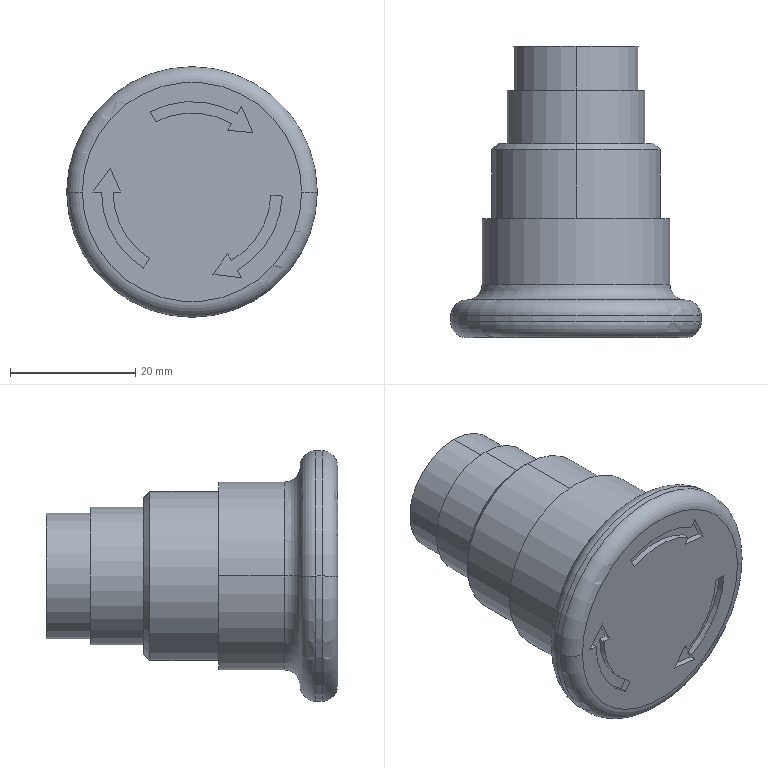Part | SolidWorks | features BaseBody 1 | 1 solid | 50 faces | box 40 x 46.5 x 40 mm | volume 27930 mm3 | plane 24 | cylinder 18 | torus 6 | cone 2 | commonest cylinder face diameters 25.213 x3 28.872 x3 18 x2 20 x2 22 x2 27 x2
STEP:
#1=CARTESIAN_POINT('',(14.421,1.,-0.6518));
#2=VERTEX_POINT('',#1);
#3=CARTESIAN_POINT('',(12.594,1.,-0.5692));
#4=VERTEX_POINT('',#3);
#5=CARTESIAN_POINT('',(14.421,1.,-0.6518));
#6=DIRECTION('',(-0.999,0.,0.04515));
#7=VECTOR('',#6,1000.);
#8=LINE('',#5,#7);
#9=EDGE_CURVE('',#2,#4,#8,.T.);
#10=ORIENTED_EDGE('',*,*,#9,.T.);
#11=CARTESIAN_POINT('',(6.303,1.,-10.918));
#12=VERTEX_POINT('',#11);
#13=CARTESIAN_POINT('',(0.,1.,0.));
#14=DIRECTION('',(0.,1.,0.));
#15=DIRECTION('',(0.999,0.,-0.04515));
#16=AXIS2_PLACEMENT_3D('',#13,#14,#15);
#17=CIRCLE('',#16,12.607);
#18=EDGE_CURVE('',#4,#12,#17,.T.);
#19=ORIENTED_EDGE('',*,*,#18,.T.);
#20=CARTESIAN_POINT('',(5.687,1.,-9.849));
#21=VERTEX_POINT('',#20);
#22=CARTESIAN_POINT('',(6.303,1.,-10.918));
#23=DIRECTION('',(-0.5,0.,0.866));
#24=VECTOR('',#23,1000.);
#25=LINE('',#22,#24);
#26=EDGE_CURVE('',#12,#21,#25,.T.);
#27=ORIENTED_EDGE('',*,*,#26,.T.);
#28=CARTESIAN_POINT('',(3.346,1.,-13.147));
#29=VERTEX_POINT('',#28);
#30=CARTESIAN_POINT('',(5.687,1.,-9.849));
#31=DIRECTION('',(-0.5788,0.,-0.8155));
#32=VECTOR('',#31,1000.);
#33=LINE('',#30,#32);
#34=EDGE_CURVE('',#21,#29,#33,.T.);
#35=ORIENTED_EDGE('',*,*,#34,.T.);
#36=CARTESIAN_POINT('',(7.903,1.,-13.688));
#37=VERTEX_POINT('',#36);
#38=CARTESIAN_POINT('',(3.346,1.,-13.147));
#39=DIRECTION('',(0.993,0.,-0.1179));
#40=VECTOR('',#39,1000.);
#41=LINE('',#38,#40);
#42=EDGE_CURVE('',#29,#37,#41,.T.);
#43=ORIENTED_EDGE('',*,*,#42,.T.);
#44=CARTESIAN_POINT('',(7.218,1.,-12.502));
#45=VERTEX_POINT('',#44);
#46=CARTESIAN_POINT('',(7.903,1.,-13.688));
#47=DIRECTION('',(-0.5,0.,0.866));
#48=VECTOR('',#47,1000.);
#49=LINE('',#46,#48);
#50=EDGE_CURVE('',#37,#45,#49,.T.);
#51=ORIENTED_EDGE('',*,*,#50,.T.);
#52=CARTESIAN_POINT('',(0.,1.,0.));
#53=DIRECTION('',(0.,-1.,0.));
#54=DIRECTION('',(0.5,0.,-0.866));
#55=AXIS2_PLACEMENT_3D('',#52,#53,#54);
#56=CIRCLE('',#55,14.436);
#57=EDGE_CURVE('',#45,#2,#56,.T.);
#58=ORIENTED_EDGE('',*,*,#57,.T.);
#59=EDGE_LOOP('',(#10,#19,#27,#35,#43,#51,#58));
#60=FACE_OUTER_BOUND('',#59,.T.);
#61=CARTESIAN_POINT('',(0.,1.,0.));
#62=DIRECTION('',(0.,-1.,0.));
#63=DIRECTION('',(-0.866,0.,-0.5));
#64=AXIS2_PLACEMENT_3D('',#61,#62,#63);
#65=PLANE('',#64);
#66=ADVANCED_FACE('',(#60),#65,.T.);
#67=CARTESIAN_POINT('',(12.594,0.,-0.5692));
#68=VERTEX_POINT('',#67);
#69=CARTESIAN_POINT('',(12.594,0.,-0.5692));
#70=DIRECTION('',(0.,1.,0.));
#71=VECTOR('',#70,1000.);
#72=LINE('',#69,#71);
#73=EDGE_CURVE('',#68,#4,#72,.T.);
#74=ORIENTED_EDGE('',*,*,#73,.T.);
#75=ORIENTED_EDGE('',*,*,#9,.F.);
#76=CARTESIAN_POINT('',(14.421,0.,-0.6518));
#77=VERTEX_POINT('',#76);
#78=CARTESIAN_POINT('',(14.421,0.,-0.6518));
#79=DIRECTION('',(0.,1.,0.));
#80=VECTOR('',#79,1000.);
#81=LINE('',#78,#80);
#82=EDGE_CURVE('',#77,#2,#81,.T.);
#83=ORIENTED_EDGE('',*,*,#82,.F.);
#84=CARTESIAN_POINT('',(14.421,0.,-0.6518));
#85=DIRECTION('',(-0.999,0.,0.04515));
#86=VECTOR('',#85,1000.);
#87=LINE('',#84,#86);
#88=EDGE_CURVE('',#77,#68,#87,.T.);
#89=ORIENTED_EDGE('',*,*,#88,.T.);
#90=EDGE_LOOP('',(#74,#75,#83,#89));
#91=FACE_OUTER_BOUND('',#90,.T.);
#92=CARTESIAN_POINT('',(14.421,0.,-0.6518));
#93=DIRECTION('',(0.04515,0.,0.999));
#94=DIRECTION('',(-0.999,0.,0.04515));
#95=AXIS2_PLACEMENT_3D('',#92,#93,#94);
#96=PLANE('',#95);
#97=ADVANCED_FACE('',(#91),#96,.F.);
#98=CARTESIAN_POINT('',(6.303,0.,-10.918));
#99=VERTEX_POINT('',#98);
#100=CARTESIAN_POINT('',(6.303,0.,-10.918));
#101=DIRECTION('',(0.,1.,0.));
#102=VECTOR('',#101,1000.);
#103=LINE('',#100,#102);
#104=EDGE_CURVE('',#99,#12,#103,.T.);
#105=ORIENTED_EDGE('',*,*,#104,.T.);
#106=ORIENTED_EDGE('',*,*,#18,.F.);
#107=ORIENTED_EDGE('',*,*,#73,.F.);
#108=CARTESIAN_POINT('',(0.,0.,0.));
#109=DIRECTION('',(0.,-1.,0.));
#110=DIRECTION('',(0.5,0.,-0.866));
#111=AXIS2_PLACEMENT_3D('',#108,#109,#110);
#112=CIRCLE('',#111,12.607);
#113=EDGE_CURVE('',#99,#68,#112,.T.);
#114=ORIENTED_EDGE('',*,*,#113,.F.);
#115=EDGE_LOOP('',(#105,#106,#107,#114));
#116=FACE_OUTER_BOUND('',#115,.T.);
#117=CARTESIAN_POINT('',(0.,0.,0.));
#118=DIRECTION('',(0.,-1.,0.));
#119=DIRECTION('',(-0.866,0.,-0.5));
#120=AXIS2_PLACEMENT_3D('',#117,#118,#119);
#121=CYLINDRICAL_SURFACE('',#120,12.607);
#122=ADVANCED_FACE('',(#116),#121,.T.);
#123=CARTESIAN_POINT('',(5.687,0.,-9.849));
#124=VERTEX_POINT('',#123);
#125=CARTESIAN_POINT('',(5.687,0.,-9.849));
#126=DIRECTION('',(0.,1.,0.));
#127=VECTOR('',#126,1000.);
#128=LINE('',#125,#127);
#129=EDGE_CURVE('',#124,#21,#128,.T.);
#130=ORIENTED_EDGE('',*,*,#129,.T.);
#131=ORIENTED_EDGE('',*,*,#26,.F.);
#132=ORIENTED_EDGE('',*,*,#104,.F.);
#133=CARTESIAN_POINT('',(6.303,0.,-10.918));
#134=DIRECTION('',(-0.5,0.,0.866));
#135=VECTOR('',#134,1000.);
#136=LINE('',#133,#135);
#137=EDGE_CURVE('',#99,#124,#136,.T.);
#138=ORIENTED_EDGE('',*,*,#137,.T.);
#139=EDGE_LOOP('',(#130,#131,#132,#138));
#140=FACE_OUTER_BOUND('',#139,.T.);
#141=CARTESIAN_POINT('',(6.303,0.,-10.918));
#142=DIRECTION('',(0.866,0.,0.5));
#143=DIRECTION('',(-0.5,0.,0.866));
#144=AXIS2_PLACEMENT_3D('',#141,#142,#143);
#145=PLANE('',#144);
#146=ADVANCED_FACE('',(#140),#145,.F.);
#147=CARTESIAN_POINT('',(3.346,0.,-13.147));
#148=VERTEX_POINT('',#147);
#149=CARTESIAN_POINT('',(3.346,0.,-13.147));
#150=DIRECTION('',(0.,1.,0.));
#151=VECTOR('',#150,1000.);
#152=LINE('',#149,#151);
#153=EDGE_CURVE('',#148,#29,#152,.T.);
#154=ORIENTED_EDGE('',*,*,#153,.T.);
#155=ORIENTED_EDGE('',*,*,#34,.F.);
#156=ORIENTED_EDGE('',*,*,#129,.F.);
#157=CARTESIAN_POINT('',(5.687,0.,-9.849));
#158=DIRECTION('',(-0.5788,0.,-0.8155));
#159=VECTOR('',#158,1000.);
#160=LINE('',#157,#159);
#161=EDGE_CURVE('',#124,#148,#160,.T.);
#162=ORIENTED_EDGE('',*,*,#161,.T.);
#163=EDGE_LOOP('',(#154,#155,#156,#162));
#164=FACE_OUTER_BOUND('',#163,.T.);
#165=CARTESIAN_POINT('',(5.687,0.,-9.849));
#166=DIRECTION('',(-0.8155,0.,0.5788));
#167=DIRECTION('',(-0.5788,0.,-0.8155));
#168=AXIS2_PLACEMENT_3D('',#165,#166,#167);
#169=PLANE('',#168);
#170=ADVANCED_FACE('',(#164),#169,.F.);
#171=CARTESIAN_POINT('',(7.903,0.,-13.688));
#172=VERTEX_POINT('',#171);
#173=CARTESIAN_POINT('',(7.903,0.,-13.688));
#174=DIRECTION('',(0.,1.,0.));
#175=VECTOR('',#174,1000.);
#176=LINE('',#173,#175);
#177=EDGE_CURVE('',#172,#37,#176,.T.);
#178=ORIENTED_EDGE('',*,*,#177,.T.);
#179=ORIENTED_EDGE('',*,*,#42,.F.);
#180=ORIENTED_EDGE('',*,*,#153,.F.);
#181=CARTESIAN_POINT('',(3.346,0.,-13.147));
#182=DIRECTION('',(0.993,0.,-0.1179));
#183=VECTOR('',#182,1000.);
#184=LINE('',#181,#183);
#185=EDGE_CURVE('',#148,#172,#184,.T.);
#186=ORIENTED_EDGE('',*,*,#185,.T.);
#187=EDGE_LOOP('',(#178,#179,#180,#186));
#188=FACE_OUTER_BOUND('',#187,.T.);
#189=CARTESIAN_POINT('',(3.346,0.,-13.147));
#190=DIRECTION('',(-0.1179,0.,-0.993));
#191=DIRECTION('',(0.993,0.,-0.1179));
#192=AXIS2_PLACEMENT_3D('',#189,#190,#191);
#193=PLANE('',#192);
#194=ADVANCED_FACE('',(#188),#193,.F.);
#195=CARTESIAN_POINT('',(7.218,0.,-12.502));
#196=VERTEX_POINT('',#195);
#197=CARTESIAN_POINT('',(7.218,0.,-12.502));
#198=DIRECTION('',(0.,1.,0.));
#199=VECTOR('',#198,1000.);
#200=LINE('',#197,#199);
#201=EDGE_CURVE('',#196,#45,#200,.T.);
#202=ORIENTED_EDGE('',*,*,#201,.T.);
#203=ORIENTED_EDGE('',*,*,#50,.F.);
#204=ORIENTED_EDGE('',*,*,#177,.F.);
#205=CARTESIAN_POINT('',(7.903,0.,-13.688));
#206=DIRECTION('',(-0.5,0.,0.866));
#207=VECTOR('',#206,1000.);
#208=LINE('',#205,#207);
#209=EDGE_CURVE('',#172,#196,#208,.T.);
#210=ORIENTED_EDGE('',*,*,#209,.T.);
#211=EDGE_LOOP('',(#202,#203,#204,#210));
#212=FACE_OUTER_BOUND('',#211,.T.);
#213=CARTESIAN_POINT('',(7.903,0.,-13.688));
#214=DIRECTION('',(0.866,0.,0.5));
#215=DIRECTION('',(-0.5,0.,0.866));
#216=AXIS2_PLACEMENT_3D('',#213,#214,#215);
#217=PLANE('',#216);
#218=ADVANCED_FACE('',(#212),#217,.F.);
#219=ORIENTED_EDGE('',*,*,#82,.T.);
#220=ORIENTED_EDGE('',*,*,#57,.F.);
#221=ORIENTED_EDGE('',*,*,#201,.F.);
#222=CARTESIAN_POINT('',(0.,0.,0.));
#223=DIRECTION('',(0.,-1.,0.));
#224=DIRECTION('',(0.5,0.,-0.866));
#225=AXIS2_PLACEMENT_3D('',#222,#223,#224);
#226=CIRCLE('',#225,14.436);
#227=EDGE_CURVE('',#196,#77,#226,.T.);
#228=ORIENTED_EDGE('',*,*,#227,.T.);
#229=EDGE_LOOP('',(#219,#220,#221,#228));
#230=FACE_OUTER_BOUND('',#229,.T.);
#231=CARTESIAN_POINT('',(0.,0.,0.));
#232=DIRECTION('',(0.,-1.,0.));
#233=DIRECTION('',(-0.866,0.,-0.5));
#234=AXIS2_PLACEMENT_3D('',#231,#232,#233);
#235=CYLINDRICAL_SURFACE('',#234,14.436);
#236=ADVANCED_FACE('',(#230),#235,.F.);
#237=CARTESIAN_POINT('',(-6.646,1.,12.815));
#238=VERTEX_POINT('',#237);
#239=CARTESIAN_POINT('',(-5.804,1.,11.191));
#240=VERTEX_POINT('',#239);
#241=CARTESIAN_POINT('',(-6.646,1.,12.815));
#242=DIRECTION('',(0.4604,0.,-0.8877));
#243=VECTOR('',#242,1000.);
#244=LINE('',#241,#243);
#245=EDGE_CURVE('',#238,#240,#244,.T.);
#246=ORIENTED_EDGE('',*,*,#245,.T.);
#247=CARTESIAN_POINT('',(6.303,1.,10.918));
#248=VERTEX_POINT('',#247);
#249=CARTESIAN_POINT('',(0.,1.,0.));
#250=DIRECTION('',(0.,1.,0.));
#251=DIRECTION('',(-0.4604,0.,0.8877));
#252=AXIS2_PLACEMENT_3D('',#249,#250,#251);
#253=CIRCLE('',#252,12.607);
#254=EDGE_CURVE('',#240,#248,#253,.T.);
#255=ORIENTED_EDGE('',*,*,#254,.T.);
#256=CARTESIAN_POINT('',(5.687,1.,9.849));
#257=VERTEX_POINT('',#256);
#258=CARTESIAN_POINT('',(6.303,1.,10.918));
#259=DIRECTION('',(-0.5,0.,-0.866));
#260=VECTOR('',#259,1000.);
#261=LINE('',#258,#260);
#262=EDGE_CURVE('',#248,#257,#261,.T.);
#263=ORIENTED_EDGE('',*,*,#262,.T.);
#264=CARTESIAN_POINT('',(9.712,1.,9.471));
#265=VERTEX_POINT('',#264);
#266=CARTESIAN_POINT('',(5.687,1.,9.849));
#267=DIRECTION('',(0.9956,0.,-0.09348));
#268=VECTOR('',#267,1000.);
#269=LINE('',#266,#268);
#270=EDGE_CURVE('',#257,#265,#269,.T.);
#271=ORIENTED_EDGE('',*,*,#270,.T.);
#272=CARTESIAN_POINT('',(7.903,1.,13.688));
#273=VERTEX_POINT('',#272);
#274=CARTESIAN_POINT('',(9.712,1.,9.471));
#275=DIRECTION('',(-0.3944,0.,0.9189));
#276=VECTOR('',#275,1000.);
#277=LINE('',#274,#276);
#278=EDGE_CURVE('',#265,#273,#277,.T.);
#279=ORIENTED_EDGE('',*,*,#278,.T.);
#280=CARTESIAN_POINT('',(7.218,1.,12.502));
#281=VERTEX_POINT('',#280);
#282=CARTESIAN_POINT('',(7.903,1.,13.688));
#283=DIRECTION('',(-0.5,0.,-0.866));
#284=VECTOR('',#283,1000.);
#285=LINE('',#282,#284);
#286=EDGE_CURVE('',#273,#281,#285,.T.);
#287=ORIENTED_EDGE('',*,*,#286,.T.);
#288=CARTESIAN_POINT('',(0.,1.,0.));
#289=DIRECTION('',(0.,-1.,0.));
#290=DIRECTION('',(0.5,0.,0.866));
#291=AXIS2_PLACEMENT_3D('',#288,#289,#290);
#292=CIRCLE('',#291,14.436);
#293=EDGE_CURVE('',#281,#238,#292,.T.);
#294=ORIENTED_EDGE('',*,*,#293,.T.);
#295=EDGE_LOOP('',(#246,#255,#263,#271,#279,#287,#294));
#296=FACE_OUTER_BOUND('',#295,.T.);
#297=CARTESIAN_POINT('',(0.,1.,0.));
#298=DIRECTION('',(0.,-1.,0.));
#299=DIRECTION('',(0.866,0.,-0.5));
#300=AXIS2_PLACEMENT_3D('',#297,#298,#299);
#301=PLANE('',#300);
#302=ADVANCED_FACE('',(#296),#301,.T.);
#303=CARTESIAN_POINT('',(-5.804,0.,11.191));
#304=VERTEX_POINT('',#303);
#305=CARTESIAN_POINT('',(-5.804,0.,11.191));
#306=DIRECTION('',(0.,1.,0.));
#307=VECTOR('',#306,1000.);
#308=LINE('',#305,#307);
#309=EDGE_CURVE('',#304,#240,#308,.T.);
#310=ORIENTED_EDGE('',*,*,#309,.T.);
#311=ORIENTED_EDGE('',*,*,#245,.F.);
#312=CARTESIAN_POINT('',(-6.646,0.,12.815));
#313=VERTEX_POINT('',#312);
#314=CARTESIAN_POINT('',(-6.646,0.,12.815));
#315=DIRECTION('',(0.,1.,0.));
#316=VECTOR('',#315,1000.);
#317=LINE('',#314,#316);
#318=EDGE_CURVE('',#313,#238,#317,.T.);
#319=ORIENTED_EDGE('',*,*,#318,.F.);
#320=CARTESIAN_POINT('',(-6.646,0.,12.815));
#321=DIRECTION('',(0.4604,0.,-0.8877));
#322=VECTOR('',#321,1000.);
#323=LINE('',#320,#322);
#324=EDGE_CURVE('',#313,#304,#323,.T.);
#325=ORIENTED_EDGE('',*,*,#324,.T.);
#326=EDGE_LOOP('',(#310,#311,#319,#325));
#327=FACE_OUTER_BOUND('',#326,.T.);
#328=CARTESIAN_POINT('',(-6.646,0.,12.815));
#329=DIRECTION('',(-0.8877,0.,-0.4604));
#330=DIRECTION('',(0.4604,0.,-0.8877));
#331=AXIS2_PLACEMENT_3D('',#328,#329,#330);
#332=PLANE('',#331);
#333=ADVANCED_FACE('',(#327),#332,.F.);
#334=CARTESIAN_POINT('',(6.303,0.,10.918));
#335=VERTEX_POINT('',#334);
#336=CARTESIAN_POINT('',(6.303,0.,10.918));
#337=DIRECTION('',(0.,1.,0.));
#338=VECTOR('',#337,1000.);
#339=LINE('',#336,#338);
#340=EDGE_CURVE('',#335,#248,#339,.T.);
#341=ORIENTED_EDGE('',*,*,#340,.T.);
#342=ORIENTED_EDGE('',*,*,#254,.F.);
#343=ORIENTED_EDGE('',*,*,#309,.F.);
#344=CARTESIAN_POINT('',(0.,0.,0.));
#345=DIRECTION('',(0.,-1.,0.));
#346=DIRECTION('',(0.5,0.,0.866));
#347=AXIS2_PLACEMENT_3D('',#344,#345,#346);
#348=CIRCLE('',#347,12.607);
#349=EDGE_CURVE('',#335,#304,#348,.T.);
#350=ORIENTED_EDGE('',*,*,#349,.F.);
#351=EDGE_LOOP('',(#341,#342,#343,#350));
#352=FACE_OUTER_BOUND('',#351,.T.);
#353=CARTESIAN_POINT('',(0.,0.,0.));
#354=DIRECTION('',(0.,-1.,0.));
#355=DIRECTION('',(0.866,0.,-0.5));
#356=AXIS2_PLACEMENT_3D('',#353,#354,#355);
#357=CYLINDRICAL_SURFACE('',#356,12.607);
#358=ADVANCED_FACE('',(#352),#357,.T.);
#359=CARTESIAN_POINT('',(5.687,0.,9.849));
#360=VERTEX_POINT('',#359);
#361=CARTESIAN_POINT('',(5.687,0.,9.849));
#362=DIRECTION('',(0.,1.,0.));
#363=VECTOR('',#362,1000.);
#364=LINE('',#361,#363);
#365=EDGE_CURVE('',#360,#257,#364,.T.);
#366=ORIENTED_EDGE('',*,*,#365,.T.);
#367=ORIENTED_EDGE('',*,*,#262,.F.);
#368=ORIENTED_EDGE('',*,*,#340,.F.);
#369=CARTESIAN_POINT('',(6.303,0.,10.918));
#370=DIRECTION('',(-0.5,0.,-0.866));
#371=VECTOR('',#370,1000.);
#372=LINE('',#369,#371);
#373=EDGE_CURVE('',#335,#360,#372,.T.);
#374=ORIENTED_EDGE('',*,*,#373,.T.);
#375=EDGE_LOOP('',(#366,#367,#368,#374));
#376=FACE_OUTER_BOUND('',#375,.T.);
#377=CARTESIAN_POINT('',(6.303,0.,10.918));
#378=DIRECTION('',(-0.866,0.,0.5));
#379=DIRECTION('',(-0.5,0.,-0.866));
#380=AXIS2_PLACEMENT_3D('',#377,#378,#379);
#381=PLANE('',#380);
#382=ADVANCED_FACE('',(#376),#381,.F.);
#383=CARTESIAN_POINT('',(9.712,0.,9.471));
#384=VERTEX_POINT('',#383);
#385=CARTESIAN_POINT('',(9.712,0.,9.471));
#386=DIRECTION('',(0.,1.,0.));
#387=VECTOR('',#386,1000.);
#388=LINE('',#385,#387);
#389=EDGE_CURVE('',#384,#265,#388,.T.);
#390=ORIENTED_EDGE('',*,*,#389,.T.);
#391=ORIENTED_EDGE('',*,*,#270,.F.);
#392=ORIENTED_EDGE('',*,*,#365,.F.);
#393=CARTESIAN_POINT('',(5.687,0.,9.849));
#394=DIRECTION('',(0.9956,0.,-0.09348));
#395=VECTOR('',#394,1000.);
#396=LINE('',#393,#395);
#397=EDGE_CURVE('',#360,#384,#396,.T.);
#398=ORIENTED_EDGE('',*,*,#397,.T.);
#399=EDGE_LOOP('',(#390,#391,#392,#398));
#400=FACE_OUTER_BOUND('',#399,.T.);
#401=CARTESIAN_POINT('',(5.687,0.,9.849));
#402=DIRECTION('',(-0.09348,0.,-0.9956));
#403=DIRECTION('',(0.9956,0.,-0.09348));
#404=AXIS2_PLACEMENT_3D('',#401,#402,#403);
#405=PLANE('',#404);
#406=ADVANCED_FACE('',(#400),#405,.F.);
#407=CARTESIAN_POINT('',(7.903,0.,13.688));
#408=VERTEX_POINT('',#407);
#409=CARTESIAN_POINT('',(7.903,0.,13.688));
#410=DIRECTION('',(0.,1.,0.));
#411=VECTOR('',#410,1000.);
#412=LINE('',#409,#411);
#413=EDGE_CURVE('',#408,#273,#412,.T.);
#414=ORIENTED_EDGE('',*,*,#413,.T.);
#415=ORIENTED_EDGE('',*,*,#278,.F.);
#416=ORIENTED_EDGE('',*,*,#389,.F.);
#417=CARTESIAN_POINT('',(9.712,0.,9.471));
#418=DIRECTION('',(-0.3944,0.,0.9189));
#419=VECTOR('',#418,1000.);
#420=LINE('',#417,#419);
#421=EDGE_CURVE('',#384,#408,#420,.T.);
#422=ORIENTED_EDGE('',*,*,#421,.T.);
#423=EDGE_LOOP('',(#414,#415,#416,#422));
#424=FACE_OUTER_BOUND('',#423,.T.);
#425=CARTESIAN_POINT('',(9.712,0.,9.471));
#426=DIRECTION('',(0.9189,0.,0.3944));
#427=DIRECTION('',(-0.3944,0.,0.9189));
#428=AXIS2_PLACEMENT_3D('',#425,#426,#427);
#429=PLANE('',#428);
#430=ADVANCED_FACE('',(#424),#429,.F.);
#431=CARTESIAN_POINT('',(7.218,0.,12.502));
#432=VERTEX_POINT('',#431);
#433=CARTESIAN_POINT('',(7.218,0.,12.502));
#434=DIRECTION('',(0.,1.,0.));
#435=VECTOR('',#434,1000.);
#436=LINE('',#433,#435);
#437=EDGE_CURVE('',#432,#281,#436,.T.);
#438=ORIENTED_EDGE('',*,*,#437,.T.);
#439=ORIENTED_EDGE('',*,*,#286,.F.);
#440=ORIENTED_EDGE('',*,*,#413,.F.);
#441=CARTESIAN_POINT('',(7.903,0.,13.688));
#442=DIRECTION('',(-0.5,0.,-0.866));
#443=VECTOR('',#442,1000.);
#444=LINE('',#441,#443);
#445=EDGE_CURVE('',#408,#432,#444,.T.);
#446=ORIENTED_EDGE('',*,*,#445,.T.);
#447=EDGE_LOOP('',(#438,#439,#440,#446));
#448=FACE_OUTER_BOUND('',#447,.T.);
#449=CARTESIAN_POINT('',(7.903,0.,13.688));
#450=DIRECTION('',(-0.866,0.,0.5));
#451=DIRECTION('',(-0.5,0.,-0.866));
#452=AXIS2_PLACEMENT_3D('',#449,#450,#451);
#453=PLANE('',#452);
#454=ADVANCED_FACE('',(#448),#453,.F.);
#455=ORIENTED_EDGE('',*,*,#318,.T.);
#456=ORIENTED_EDGE('',*,*,#293,.F.);
#457=ORIENTED_EDGE('',*,*,#437,.F.);
#458=CARTESIAN_POINT('',(0.,0.,0.));
#459=DIRECTION('',(0.,-1.,0.));
#460=DIRECTION('',(0.5,0.,0.866));
#461=AXIS2_PLACEMENT_3D('',#458,#459,#460);
#462=CIRCLE('',#461,14.436);
#463=EDGE_CURVE('',#432,#313,#462,.T.);
#464=ORIENTED_EDGE('',*,*,#463,.T.);
#465=EDGE_LOOP('',(#455,#456,#457,#464));
#466=FACE_OUTER_BOUND('',#465,.T.);
#467=CARTESIAN_POINT('',(0.,0.,0.));
#468=DIRECTION('',(0.,-1.,0.));
#469=DIRECTION('',(0.866,0.,-0.5));
#470=AXIS2_PLACEMENT_3D('',#467,#468,#469);
#471=CYLINDRICAL_SURFACE('',#470,14.436);
#472=ADVANCED_FACE('',(#466),#471,.F.);
#473=CARTESIAN_POINT('',(-7.775,1.,-12.163));
#474=VERTEX_POINT('',#473);
#475=CARTESIAN_POINT('',(-6.79,1.,-10.622));
#476=VERTEX_POINT('',#475);
#477=CARTESIAN_POINT('',(-7.775,1.,-12.163));
#478=DIRECTION('',(0.5386,0.,0.8426));
#479=VECTOR('',#478,1000.);
#480=LINE('',#477,#479);
#481=EDGE_CURVE('',#474,#476,#480,.T.);
#482=ORIENTED_EDGE('',*,*,#481,.T.);
#483=CARTESIAN_POINT('',(-12.607,1.,0.));
#484=VERTEX_POINT('',#483);
#485=CARTESIAN_POINT('',(0.,1.,0.));
#486=DIRECTION('',(0.,1.,0.));
#487=DIRECTION('',(-0.5386,0.,-0.8426));
#488=AXIS2_PLACEMENT_3D('',#485,#486,#487);
#489=CIRCLE('',#488,12.607);
#490=EDGE_CURVE('',#476,#484,#489,.T.);
#491=ORIENTED_EDGE('',*,*,#490,.T.);
#492=CARTESIAN_POINT('',(-11.373,1.,0.));
#493=VERTEX_POINT('',#492);
#494=CARTESIAN_POINT('',(-12.607,1.,0.));
#495=DIRECTION('',(1.,0.,0.));
#496=VECTOR('',#495,1000.);
#497=LINE('',#494,#496);
#498=EDGE_CURVE('',#484,#493,#497,.T.);
#499=ORIENTED_EDGE('',*,*,#498,.T.);
#500=CARTESIAN_POINT('',(-13.059,1.,3.675));
#501=VERTEX_POINT('',#500);
#502=CARTESIAN_POINT('',(-11.373,1.,0.));
#503=DIRECTION('',(-0.4169,0.,0.909));
#504=VECTOR('',#503,1000.);
#505=LINE('',#502,#504);
#506=EDGE_CURVE('',#493,#501,#505,.T.);
#507=ORIENTED_EDGE('',*,*,#506,.T.);
#508=CARTESIAN_POINT('',(-15.805,1.,0.));
#509=VERTEX_POINT('',#508);
#510=CARTESIAN_POINT('',(-13.059,1.,3.675));
#511=DIRECTION('',(-0.5986,0.,-0.801));
#512=VECTOR('',#511,1000.);
#513=LINE('',#510,#512);
#514=EDGE_CURVE('',#501,#509,#513,.T.);
#515=ORIENTED_EDGE('',*,*,#514,.T.);
#516=CARTESIAN_POINT('',(-14.436,1.,0.));
#517=VERTEX_POINT('',#516);
#518=CARTESIAN_POINT('',(-15.805,1.,0.));
#519=DIRECTION('',(1.,0.,0.));
#520=VECTOR('',#519,1000.);
#521=LINE('',#518,#520);
#522=EDGE_CURVE('',#509,#517,#521,.T.);
#523=ORIENTED_EDGE('',*,*,#522,.T.);
#524=CARTESIAN_POINT('',(0.,1.,0.));
#525=DIRECTION('',(0.,-1.,0.));
#526=DIRECTION('',(-1.,0.,0.));
#527=AXIS2_PLACEMENT_3D('',#524,#525,#526);
#528=CIRCLE('',#527,14.436);
#529=EDGE_CURVE('',#517,#474,#528,.T.);
#530=ORIENTED_EDGE('',*,*,#529,.T.);
#531=EDGE_LOOP('',(#482,#491,#499,#507,#515,#523,#530));
#532=FACE_OUTER_BOUND('',#531,.T.);
#533=CARTESIAN_POINT('',(0.,1.,0.));
#534=DIRECTION('',(0.,-1.,0.));
#535=DIRECTION('',(0.,0.,1.));
#536=AXIS2_PLACEMENT_3D('',#533,#534,#535);
#537=PLANE('',#536);
#538=ADVANCED_FACE('',(#532),#537,.T.);
#539=CARTESIAN_POINT('',(-6.79,0.,-10.622));
#540=VERTEX_POINT('',#539);
#541=CARTESIAN_POINT('',(-6.79,0.,-10.622));
#542=DIRECTION('',(0.,1.,0.));
#543=VECTOR('',#542,1000.);
#544=LINE('',#541,#543);
#545=EDGE_CURVE('',#540,#476,#544,.T.);
#546=ORIENTED_EDGE('',*,*,#545,.T.);
#547=ORIENTED_EDGE('',*,*,#481,.F.);
#548=CARTESIAN_POINT('',(-7.775,0.,-12.163));
#549=VERTEX_POINT('',#548);
#550=CARTESIAN_POINT('',(-7.775,0.,-12.163));
#551=DIRECTION('',(0.,1.,0.));
#552=VECTOR('',#551,1000.);
#553=LINE('',#550,#552);
#554=EDGE_CURVE('',#549,#474,#553,.T.);
#555=ORIENTED_EDGE('',*,*,#554,.F.);
#556=CARTESIAN_POINT('',(-7.775,0.,-12.163));
#557=DIRECTION('',(0.5386,0.,0.8426));
#558=VECTOR('',#557,1000.);
#559=LINE('',#556,#558);
#560=EDGE_CURVE('',#549,#540,#559,.T.);
#561=ORIENTED_EDGE('',*,*,#560,.T.);
#562=EDGE_LOOP('',(#546,#547,#555,#561));
#563=FACE_OUTER_BOUND('',#562,.T.);
#564=CARTESIAN_POINT('',(-7.775,0.,-12.163));
#565=DIRECTION('',(0.8426,0.,-0.5386));
#566=DIRECTION('',(0.5386,0.,0.8426));
#567=AXIS2_PLACEMENT_3D('',#564,#565,#566);
#568=PLANE('',#567);
#569=ADVANCED_FACE('',(#563),#568,.F.);
#570=CARTESIAN_POINT('',(-12.607,0.,0.));
#571=VERTEX_POINT('',#570);
#572=CARTESIAN_POINT('',(-12.607,0.,0.));
#573=DIRECTION('',(0.,1.,0.));
#574=VECTOR('',#573,1000.);
#575=LINE('',#572,#574);
#576=EDGE_CURVE('',#571,#484,#575,.T.);
#577=ORIENTED_EDGE('',*,*,#576,.T.);
#578=ORIENTED_EDGE('',*,*,#490,.F.);
#579=ORIENTED_EDGE('',*,*,#545,.F.);
#580=CARTESIAN_POINT('',(0.,0.,0.));
#581=DIRECTION('',(0.,-1.,0.));
#582=DIRECTION('',(-1.,0.,0.));
#583=AXIS2_PLACEMENT_3D('',#580,#581,#582);
#584=CIRCLE('',#583,12.607);
#585=EDGE_CURVE('',#571,#540,#584,.T.);
#586=ORIENTED_EDGE('',*,*,#585,.F.);
#587=EDGE_LOOP('',(#577,#578,#579,#586));
#588=FACE_OUTER_BOUND('',#587,.T.);
#589=CARTESIAN_POINT('',(0.,0.,0.));
#590=DIRECTION('',(0.,-1.,0.));
#591=DIRECTION('',(0.,0.,1.));
#592=AXIS2_PLACEMENT_3D('',#589,#590,#591);
#593=CYLINDRICAL_SURFACE('',#592,12.607);
#594=ADVANCED_FACE('',(#588),#593,.T.);
#595=CARTESIAN_POINT('',(-11.373,0.,0.));
#596=VERTEX_POINT('',#595);
#597=CARTESIAN_POINT('',(-11.373,0.,0.));
#598=DIRECTION('',(0.,1.,0.));
#599=VECTOR('',#598,1000.);
#600=LINE('',#597,#599);
#601=EDGE_CURVE('',#596,#493,#600,.T.);
#602=ORIENTED_EDGE('',*,*,#601,.T.);
#603=ORIENTED_EDGE('',*,*,#498,.F.);
#604=ORIENTED_EDGE('',*,*,#576,.F.);
#605=CARTESIAN_POINT('',(-12.607,0.,0.));
#606=DIRECTION('',(1.,0.,0.));
#607=VECTOR('',#606,1000.);
#608=LINE('',#605,#607);
#609=EDGE_CURVE('',#571,#596,#608,.T.);
#610=ORIENTED_EDGE('',*,*,#609,.T.);
#611=EDGE_LOOP('',(#602,#603,#604,#610));
#612=FACE_OUTER_BOUND('',#611,.T.);
#613=CARTESIAN_POINT('',(-12.607,0.,0.));
#614=DIRECTION('',(0.,0.,-1.));
#615=DIRECTION('',(1.,0.,0.));
#616=AXIS2_PLACEMENT_3D('',#613,#614,#615);
#617=PLANE('',#616);
#618=ADVANCED_FACE('',(#612),#617,.F.);
#619=CARTESIAN_POINT('',(-13.059,0.,3.675));
#620=VERTEX_POINT('',#619);
#621=CARTESIAN_POINT('',(-13.059,0.,3.675));
#622=DIRECTION('',(0.,1.,0.));
#623=VECTOR('',#622,1000.);
#624=LINE('',#621,#623);
#625=EDGE_CURVE('',#620,#501,#624,.T.);
#626=ORIENTED_EDGE('',*,*,#625,.T.);
#627=ORIENTED_EDGE('',*,*,#506,.F.);
#628=ORIENTED_EDGE('',*,*,#601,.F.);
#629=CARTESIAN_POINT('',(-11.373,0.,0.));
#630=DIRECTION('',(-0.4169,0.,0.909));
#631=VECTOR('',#630,1000.);
#632=LINE('',#629,#631);
#633=EDGE_CURVE('',#596,#620,#632,.T.);
#634=ORIENTED_EDGE('',*,*,#633,.T.);
#635=EDGE_LOOP('',(#626,#627,#628,#634));
#636=FACE_OUTER_BOUND('',#635,.T.);
#637=CARTESIAN_POINT('',(-11.373,0.,0.));
#638=DIRECTION('',(0.909,0.,0.4169));
#639=DIRECTION('',(-0.4169,0.,0.909));
#640=AXIS2_PLACEMENT_3D('',#637,#638,#639);
#641=PLANE('',#640);
#642=ADVANCED_FACE('',(#636),#641,.F.);
#643=CARTESIAN_POINT('',(-15.805,0.,0.));
#644=VERTEX_POINT('',#643);
#645=CARTESIAN_POINT('',(-15.805,0.,0.));
#646=DIRECTION('',(0.,1.,0.));
#647=VECTOR('',#646,1000.);
#648=LINE('',#645,#647);
#649=EDGE_CURVE('',#644,#509,#648,.T.);
#650=ORIENTED_EDGE('',*,*,#649,.T.);
#651=ORIENTED_EDGE('',*,*,#514,.F.);
#652=ORIENTED_EDGE('',*,*,#625,.F.);
#653=CARTESIAN_POINT('',(-13.059,0.,3.675));
#654=DIRECTION('',(-0.5986,0.,-0.801));
#655=VECTOR('',#654,1000.);
#656=LINE('',#653,#655);
#657=EDGE_CURVE('',#620,#644,#656,.T.);
#658=ORIENTED_EDGE('',*,*,#657,.T.);
#659=EDGE_LOOP('',(#650,#651,#652,#658));
#660=FACE_OUTER_BOUND('',#659,.T.);
#661=CARTESIAN_POINT('',(-13.059,0.,3.675));
#662=DIRECTION('',(-0.801,0.,0.5986));
#663=DIRECTION('',(-0.5986,0.,-0.801));
#664=AXIS2_PLACEMENT_3D('',#661,#662,#663);
#665=PLANE('',#664);
#666=ADVANCED_FACE('',(#660),#665,.F.);
#667=CARTESIAN_POINT('',(-14.436,0.,0.));
#668=VERTEX_POINT('',#667);
#669=CARTESIAN_POINT('',(-14.436,0.,0.));
#670=DIRECTION('',(0.,1.,0.));
#671=VECTOR('',#670,1000.);
#672=LINE('',#669,#671);
#673=EDGE_CURVE('',#668,#517,#672,.T.);
#674=ORIENTED_EDGE('',*,*,#673,.T.);
#675=ORIENTED_EDGE('',*,*,#522,.F.);
#676=ORIENTED_EDGE('',*,*,#649,.F.);
#677=CARTESIAN_POINT('',(-15.805,0.,0.));
#678=DIRECTION('',(1.,0.,0.));
#679=VECTOR('',#678,1000.);
#680=LINE('',#677,#679);
#681=EDGE_CURVE('',#644,#668,#680,.T.);
#682=ORIENTED_EDGE('',*,*,#681,.T.);
#683=EDGE_LOOP('',(#674,#675,#676,#682));
#684=FACE_OUTER_BOUND('',#683,.T.);
#685=CARTESIAN_POINT('',(-15.805,0.,0.));
#686=DIRECTION('',(0.,0.,-1.));
#687=DIRECTION('',(1.,0.,0.));
#688=AXIS2_PLACEMENT_3D('',#685,#686,#687);
#689=PLANE('',#688);
#690=ADVANCED_FACE('',(#684),#689,.F.);
#691=ORIENTED_EDGE('',*,*,#554,.T.);
#692=ORIENTED_EDGE('',*,*,#529,.F.);
#693=ORIENTED_EDGE('',*,*,#673,.F.);
#694=CARTESIAN_POINT('',(0.,0.,0.));
#695=DIRECTION('',(0.,-1.,0.));
#696=DIRECTION('',(-1.,0.,0.));
#697=AXIS2_PLACEMENT_3D('',#694,#695,#696);
#698=CIRCLE('',#697,14.436);
#699=EDGE_CURVE('',#668,#549,#698,.T.);
#700=ORIENTED_EDGE('',*,*,#699,.T.);
#701=EDGE_LOOP('',(#691,#692,#693,#700));
#702=FACE_OUTER_BOUND('',#701,.T.);
#703=CARTESIAN_POINT('',(0.,0.,0.));
#704=DIRECTION('',(0.,-1.,0.));
#705=DIRECTION('',(0.,0.,1.));
#706=AXIS2_PLACEMENT_3D('',#703,#704,#705);
#707=CYLINDRICAL_SURFACE('',#706,14.436);
#708=ADVANCED_FACE('',(#702),#707,.F.);
#709=CARTESIAN_POINT('',(9.,43.5,0.));
#710=VERTEX_POINT('',#709);
#711=CARTESIAN_POINT('',(-9.,43.5,0.));
#712=VERTEX_POINT('',#711);
#713=CARTESIAN_POINT('',(0.,43.5,0.));
#714=DIRECTION('',(0.,1.,0.));
#715=DIRECTION('',(1.,0.,0.));
#716=AXIS2_PLACEMENT_3D('',#713,#714,#715);
#717=CIRCLE('',#716,9.);
#718=EDGE_CURVE('',#710,#712,#717,.T.);
#719=ORIENTED_EDGE('',*,*,#718,.T.);
#720=CARTESIAN_POINT('',(0.,43.5,0.));
#721=DIRECTION('',(0.,1.,0.));
#722=DIRECTION('',(-1.,0.,0.));
#723=AXIS2_PLACEMENT_3D('',#720,#721,#722);
#724=CIRCLE('',#723,9.);
#725=EDGE_CURVE('',#712,#710,#724,.T.);
#726=ORIENTED_EDGE('',*,*,#725,.T.);
#727=EDGE_LOOP('',(#719,#726));
#728=FACE_OUTER_BOUND('',#727,.T.);
#729=CARTESIAN_POINT('',(0.,43.5,0.));
#730=DIRECTION('',(0.,1.,0.));
#731=DIRECTION('',(-1.,0.,0.));
#732=AXIS2_PLACEMENT_3D('',#729,#730,#731);
#733=PLANE('',#732);
#734=ADVANCED_FACE('',(#728),#733,.T.);
#735=CARTESIAN_POINT('',(-9.,46.5,0.));
#736=VERTEX_POINT('',#735);
#737=CARTESIAN_POINT('',(-9.,46.5,0.));
#738=DIRECTION('',(0.,-1.,0.));
#739=VECTOR('',#738,1000.);
#740=LINE('',#737,#739);
#741=EDGE_CURVE('',#736,#712,#740,.T.);
#742=ORIENTED_EDGE('',*,*,#741,.T.);
#743=ORIENTED_EDGE('',*,*,#718,.F.);
#744=CARTESIAN_POINT('',(9.,46.5,0.));
#745=VERTEX_POINT('',#744);
#746=CARTESIAN_POINT('',(9.,46.5,0.));
#747=DIRECTION('',(0.,-1.,0.));
#748=VECTOR('',#747,1000.);
#749=LINE('',#746,#748);
#750=EDGE_CURVE('',#745,#710,#749,.T.);
#751=ORIENTED_EDGE('',*,*,#750,.F.);
#752=CARTESIAN_POINT('',(0.,46.5,0.));
#753=DIRECTION('',(0.,1.,0.));
#754=DIRECTION('',(1.,0.,0.));
#755=AXIS2_PLACEMENT_3D('',#752,#753,#754);
#756=CIRCLE('',#755,9.);
#757=EDGE_CURVE('',#745,#736,#756,.T.);
#758=ORIENTED_EDGE('',*,*,#757,.T.);
#759=EDGE_LOOP('',(#742,#743,#751,#758));
#760=FACE_OUTER_BOUND('',#759,.T.);
#761=CARTESIAN_POINT('',(0.,46.5,0.));
#762=DIRECTION('',(0.,1.,0.));
#763=DIRECTION('',(-1.,0.,0.));
#764=AXIS2_PLACEMENT_3D('',#761,#762,#763);
#765=CYLINDRICAL_SURFACE('',#764,9.);
#766=ADVANCED_FACE('',(#760),#765,.F.);
#767=ORIENTED_EDGE('',*,*,#750,.T.);
#768=ORIENTED_EDGE('',*,*,#725,.F.);
#769=ORIENTED_EDGE('',*,*,#741,.F.);
#770=CARTESIAN_POINT('',(0.,46.5,0.));
#771=DIRECTION('',(0.,1.,0.));
#772=DIRECTION('',(-1.,0.,0.));
#773=AXIS2_PLACEMENT_3D('',#770,#771,#772);
#774=CIRCLE('',#773,9.);
#775=EDGE_CURVE('',#736,#745,#774,.T.);
#776=ORIENTED_EDGE('',*,*,#775,.T.);
#777=EDGE_LOOP('',(#767,#768,#769,#776));
#778=FACE_OUTER_BOUND('',#777,.T.);
#779=CARTESIAN_POINT('',(0.,46.5,0.));
#780=DIRECTION('',(0.,1.,0.));
#781=DIRECTION('',(-1.,0.,0.));
#782=AXIS2_PLACEMENT_3D('',#779,#780,#781);
#783=CYLINDRICAL_SURFACE('',#782,9.);
#784=ADVANCED_FACE('',(#778),#783,.F.);
#785=ORIENTED_EDGE('',*,*,#757,.F.);
#786=ORIENTED_EDGE('',*,*,#775,.F.);
#787=EDGE_LOOP('',(#785,#786));
#788=FACE_BOUND('',#787,.T.);
#789=CARTESIAN_POINT('',(0.,46.5,10.));
#790=VERTEX_POINT('',#789);
#791=CARTESIAN_POINT('',(0.,46.5,-10.));
#792=VERTEX_POINT('',#791);
#793=CARTESIAN_POINT('',(0.,46.5,0.));
#794=DIRECTION('',(0.,1.,0.));
#795=DIRECTION('',(0.,0.,1.));
#796=AXIS2_PLACEMENT_3D('',#793,#794,#795);
#797=CIRCLE('',#796,10.);
#798=EDGE_CURVE('',#790,#792,#797,.T.);
#799=ORIENTED_EDGE('',*,*,#798,.T.);
#800=CARTESIAN_POINT('',(0.,46.5,0.));
#801=DIRECTION('',(0.,1.,0.));
#802=DIRECTION('',(0.,0.,-1.));
#803=AXIS2_PLACEMENT_3D('',#800,#801,#802);
#804=CIRCLE('',#803,10.);
#805=EDGE_CURVE('',#792,#790,#804,.T.);
#806=ORIENTED_EDGE('',*,*,#805,.T.);
#807=EDGE_LOOP('',(#799,#806));
#808=FACE_OUTER_BOUND('',#807,.T.);
#809=CARTESIAN_POINT('',(0.,46.5,0.));
#810=DIRECTION('',(0.,1.,0.));
#811=DIRECTION('',(0.,0.,-1.));
#812=AXIS2_PLACEMENT_3D('',#809,#810,#811);
#813=PLANE('',#812);
#814=ADVANCED_FACE('',(#788,#808),#813,.T.);
#815=CARTESIAN_POINT('',(0.,39.5,-10.));
#816=VERTEX_POINT('',#815);
#817=CARTESIAN_POINT('',(0.,39.5,-10.));
#818=DIRECTION('',(0.,1.,0.));
#819=VECTOR('',#818,1000.);
#820=LINE('',#817,#819);
#821=EDGE_CURVE('',#816,#792,#820,.T.);
#822=ORIENTED_EDGE('',*,*,#821,.T.);
#823=ORIENTED_EDGE('',*,*,#798,.F.);
#824=CARTESIAN_POINT('',(0.,39.5,10.));
#825=VERTEX_POINT('',#824);
#826=CARTESIAN_POINT('',(0.,39.5,10.));
#827=DIRECTION('',(0.,1.,0.));
#828=VECTOR('',#827,1000.);
#829=LINE('',#826,#828);
#830=EDGE_CURVE('',#825,#790,#829,.T.);
#831=ORIENTED_EDGE('',*,*,#830,.F.);
#832=CARTESIAN_POINT('',(0.,39.5,0.));
#833=DIRECTION('',(0.,1.,0.));
#834=DIRECTION('',(0.,0.,1.));
#835=AXIS2_PLACEMENT_3D('',#832,#833,#834);
#836=CIRCLE('',#835,10.);
#837=EDGE_CURVE('',#825,#816,#836,.T.);
#838=ORIENTED_EDGE('',*,*,#837,.T.);
#839=EDGE_LOOP('',(#822,#823,#831,#838));
#840=FACE_OUTER_BOUND('',#839,.T.);
#841=CARTESIAN_POINT('',(0.,39.5,0.));
#842=DIRECTION('',(0.,1.,0.));
#843=DIRECTION('',(0.,0.,-1.));
#844=AXIS2_PLACEMENT_3D('',#841,#842,#843);
#845=CYLINDRICAL_SURFACE('',#844,10.);
#846=ADVANCED_FACE('',(#840),#845,.T.);
#847=ORIENTED_EDGE('',*,*,#830,.T.);
#848=ORIENTED_EDGE('',*,*,#805,.F.);
#849=ORIENTED_EDGE('',*,*,#821,.F.);
#850=CARTESIAN_POINT('',(0.,39.5,0.));
#851=DIRECTION('',(0.,1.,0.));
#852=DIRECTION('',(0.,0.,-1.));
#853=AXIS2_PLACEMENT_3D('',#850,#851,#852);
#854=CIRCLE('',#853,10.);
#855=EDGE_CURVE('',#816,#825,#854,.T.);
#856=ORIENTED_EDGE('',*,*,#855,.T.);
#857=EDGE_LOOP('',(#847,#848,#849,#856));
#858=FACE_OUTER_BOUND('',#857,.T.);
#859=CARTESIAN_POINT('',(0.,39.5,0.));
#860=DIRECTION('',(0.,1.,0.));
#861=DIRECTION('',(0.,0.,-1.));
#862=AXIS2_PLACEMENT_3D('',#859,#860,#861);
#863=CYLINDRICAL_SURFACE('',#862,10.);
#864=ADVANCED_FACE('',(#858),#863,.T.);
#865=ORIENTED_EDGE('',*,*,#837,.F.);
#866=ORIENTED_EDGE('',*,*,#855,.F.);
#867=EDGE_LOOP('',(#865,#866));
#868=FACE_BOUND('',#867,.T.);
#869=CARTESIAN_POINT('',(0.,39.5,11.));
#870=VERTEX_POINT('',#869);
#871=CARTESIAN_POINT('',(0.,39.5,-11.));
#872=VERTEX_POINT('',#871);
#873=CARTESIAN_POINT('',(0.,39.5,0.));
#874=DIRECTION('',(0.,1.,0.));
#875=DIRECTION('',(0.,0.,1.));
#876=AXIS2_PLACEMENT_3D('',#873,#874,#875);
#877=CIRCLE('',#876,11.);
#878=EDGE_CURVE('',#870,#872,#877,.T.);
#879=ORIENTED_EDGE('',*,*,#878,.T.);
#880=CARTESIAN_POINT('',(0.,39.5,0.));
#881=DIRECTION('',(0.,1.,0.));
#882=DIRECTION('',(0.,0.,-1.));
#883=AXIS2_PLACEMENT_3D('',#880,#881,#882);
#884=CIRCLE('',#883,11.);
#885=EDGE_CURVE('',#872,#870,#884,.T.);
#886=ORIENTED_EDGE('',*,*,#885,.T.);
#887=EDGE_LOOP('',(#879,#886));
#888=FACE_OUTER_BOUND('',#887,.T.);
#889=CARTESIAN_POINT('',(0.,39.5,0.));
#890=DIRECTION('',(0.,1.,0.));
#891=DIRECTION('',(0.,0.,-1.));
#892=AXIS2_PLACEMENT_3D('',#889,#890,#891);
#893=PLANE('',#892);
#894=ADVANCED_FACE('',(#868,#888),#893,.T.);
#895=CARTESIAN_POINT('',(0.,31.,-11.));
#896=VERTEX_POINT('',#895);
#897=CARTESIAN_POINT('',(0.,31.,-11.));
#898=DIRECTION('',(0.,1.,0.));
#899=VECTOR('',#898,1000.);
#900=LINE('',#897,#899);
#901=EDGE_CURVE('',#896,#872,#900,.T.);
#902=ORIENTED_EDGE('',*,*,#901,.T.);
#903=ORIENTED_EDGE('',*,*,#878,.F.);
#904=CARTESIAN_POINT('',(0.,31.,11.));
#905=VERTEX_POINT('',#904);
#906=CARTESIAN_POINT('',(0.,31.,11.));
#907=DIRECTION('',(0.,1.,0.));
#908=VECTOR('',#907,1000.);
#909=LINE('',#906,#908);
#910=EDGE_CURVE('',#905,#870,#909,.T.);
#911=ORIENTED_EDGE('',*,*,#910,.F.);
#912=CARTESIAN_POINT('',(0.,31.,0.));
#913=DIRECTION('',(0.,1.,0.));
#914=DIRECTION('',(0.,0.,1.));
#915=AXIS2_PLACEMENT_3D('',#912,#913,#914);
#916=CIRCLE('',#915,11.);
#917=EDGE_CURVE('',#905,#896,#916,.T.);
#918=ORIENTED_EDGE('',*,*,#917,.T.);
#919=EDGE_LOOP('',(#902,#903,#911,#918));
#920=FACE_OUTER_BOUND('',#919,.T.);
#921=CARTESIAN_POINT('',(0.,31.,0.));
#922=DIRECTION('',(0.,1.,0.));
#923=DIRECTION('',(0.,0.,-1.));
#924=AXIS2_PLACEMENT_3D('',#921,#922,#923);
#925=CYLINDRICAL_SURFACE('',#924,11.);
#926=ADVANCED_FACE('',(#920),#925,.T.);
#927=ORIENTED_EDGE('',*,*,#910,.T.);
#928=ORIENTED_EDGE('',*,*,#885,.F.);
#929=ORIENTED_EDGE('',*,*,#901,.F.);
#930=CARTESIAN_POINT('',(0.,31.,0.));
#931=DIRECTION('',(0.,1.,0.));
#932=DIRECTION('',(0.,0.,-1.));
#933=AXIS2_PLACEMENT_3D('',#930,#931,#932);
#934=CIRCLE('',#933,11.);
#935=EDGE_CURVE('',#896,#905,#934,.T.);
#936=ORIENTED_EDGE('',*,*,#935,.T.);
#937=EDGE_LOOP('',(#927,#928,#929,#936));
#938=FACE_OUTER_BOUND('',#937,.T.);
#939=CARTESIAN_POINT('',(0.,31.,0.));
#940=DIRECTION('',(0.,1.,0.));
#941=DIRECTION('',(0.,0.,-1.));
#942=AXIS2_PLACEMENT_3D('',#939,#940,#941);
#943=CYLINDRICAL_SURFACE('',#942,11.);
#944=ADVANCED_FACE('',(#938),#943,.T.);
#945=CARTESIAN_POINT('',(0.,19.,13.5));
#946=VERTEX_POINT('',#945);
#947=CARTESIAN_POINT('',(0.000000003,30.,13.5));
#948=VERTEX_POINT('',#947);
#949=CARTESIAN_POINT('',(0.,19.,13.5));
#950=DIRECTION('',(0.,1.,0.));
#951=VECTOR('',#950,1000.);
#952=LINE('',#949,#951);
#953=EDGE_CURVE('',#946,#948,#952,.T.);
#954=ORIENTED_EDGE('',*,*,#953,.F.);
#955=CARTESIAN_POINT('',(0.,19.,-13.5));
#956=VERTEX_POINT('',#955);
#957=CARTESIAN_POINT('',(0.,19.,0.));
#958=DIRECTION('',(0.,1.,0.));
#959=DIRECTION('',(0.,0.,1.));
#960=AXIS2_PLACEMENT_3D('',#957,#958,#959);
#961=CIRCLE('',#960,13.5);
#962=EDGE_CURVE('',#946,#956,#961,.T.);
#963=ORIENTED_EDGE('',*,*,#962,.T.);
#964=CARTESIAN_POINT('',(-0.000000003,30.,-13.5));
#965=VERTEX_POINT('',#964);
#966=CARTESIAN_POINT('',(0.,19.,-13.5));
#967=DIRECTION('',(0.,1.,0.));
#968=VECTOR('',#967,1000.);
#969=LINE('',#966,#968);
#970=EDGE_CURVE('',#956,#965,#969,.T.);
#971=ORIENTED_EDGE('',*,*,#970,.T.);
#972=CARTESIAN_POINT('',(0.,30.,0.));
#973=DIRECTION('',(0.,1.,0.));
#974=DIRECTION('',(0.,0.,1.));
#975=AXIS2_PLACEMENT_3D('',#972,#973,#974);
#976=CIRCLE('',#975,13.5);
#977=EDGE_CURVE('',#948,#965,#976,.T.);
#978=ORIENTED_EDGE('',*,*,#977,.F.);
#979=EDGE_LOOP('',(#954,#963,#971,#978));
#980=FACE_OUTER_BOUND('',#979,.T.);
#981=CARTESIAN_POINT('',(0.,19.,0.));
#982=DIRECTION('',(0.,1.,0.));
#983=DIRECTION('',(0.,0.,-1.));
#984=AXIS2_PLACEMENT_3D('',#981,#982,#983);
#985=CYLINDRICAL_SURFACE('',#984,13.5);
#986=ADVANCED_FACE('',(#980),#985,.T.);
#987=CARTESIAN_POINT('',(0.000000004,31.,12.5));
#988=VERTEX_POINT('',#987);
#989=CARTESIAN_POINT('',(-0.00000005,31.,12.5));
#990=DIRECTION('',(-0.000000003,-0.7071,0.7071));
#991=VECTOR('',#990,1000.);
#992=LINE('',#989,#991);
#993=EDGE_CURVE('',#988,#948,#992,.T.);
#994=ORIENTED_EDGE('',*,*,#993,.T.);
#995=ORIENTED_EDGE('',*,*,#977,.T.);
#996=CARTESIAN_POINT('',(-0.000000004,31.,-12.5));
#997=VERTEX_POINT('',#996);
#998=CARTESIAN_POINT('',(0.00000005,31.,-12.5));
#999=DIRECTION('',(0.000000003,-0.7071,-0.7071));
#1000=VECTOR('',#999,1000.);
#1001=LINE('',#998,#1000);
#1002=EDGE_CURVE('',#997,#965,#1001,.T.);
#1003=ORIENTED_EDGE('',*,*,#1002,.F.);
#1004=CARTESIAN_POINT('',(0.,31.,0.));
#1005=DIRECTION('',(0.,1.,0.));
#1006=DIRECTION('',(0.,0.,1.));
#1007=AXIS2_PLACEMENT_3D('',#1004,#1005,#1006);
#1008=CIRCLE('',#1007,12.5);
#1009=EDGE_CURVE('',#988,#997,#1008,.T.);
#1010=ORIENTED_EDGE('',*,*,#1009,.F.);
#1011=EDGE_LOOP('',(#994,#995,#1003,#1010));
#1012=FACE_OUTER_BOUND('',#1011,.T.);
#1013=CARTESIAN_POINT('',(0.,31.062,0.));
#1014=DIRECTION('',(0.,-1.,0.));
#1015=DIRECTION('',(0.,0.,-1.));
#1016=AXIS2_PLACEMENT_3D('',#1013,#1014,#1015);
#1017=CONICAL_SURFACE('',#1016,12.438,0.7854);
#1018=ADVANCED_FACE('',(#1012),#1017,.T.);
#1019=ORIENTED_EDGE('',*,*,#917,.F.);
#1020=ORIENTED_EDGE('',*,*,#935,.F.);
#1021=EDGE_LOOP('',(#1019,#1020));
#1022=FACE_BOUND('',#1021,.T.);
#1023=CARTESIAN_POINT('',(0.,31.,0.));
#1024=DIRECTION('',(0.,1.,0.));
#1025=DIRECTION('',(0.,0.,-1.));
#1026=AXIS2_PLACEMENT_3D('',#1023,#1024,#1025);
#1027=CIRCLE('',#1026,12.5);
#1028=EDGE_CURVE('',#997,#988,#1027,.T.);
#1029=ORIENTED_EDGE('',*,*,#1028,.T.);
#1030=ORIENTED_EDGE('',*,*,#1009,.T.);
#1031=EDGE_LOOP('',(#1029,#1030));
#1032=FACE_OUTER_BOUND('',#1031,.T.);
#1033=CARTESIAN_POINT('',(0.,31.,0.));
#1034=DIRECTION('',(0.,1.,0.));
#1035=DIRECTION('',(0.,0.,-1.));
#1036=AXIS2_PLACEMENT_3D('',#1033,#1034,#1035);
#1037=PLANE('',#1036);
#1038=ADVANCED_FACE('',(#1022,#1032),#1037,.T.);
#1039=ORIENTED_EDGE('',*,*,#1002,.T.);
#1040=CARTESIAN_POINT('',(0.,30.,0.));
#1041=DIRECTION('',(0.,1.,0.));
#1042=DIRECTION('',(0.,0.,-1.));
#1043=AXIS2_PLACEMENT_3D('',#1040,#1041,#1042);
#1044=CIRCLE('',#1043,13.5);
#1045=EDGE_CURVE('',#965,#948,#1044,.T.);
#1046=ORIENTED_EDGE('',*,*,#1045,.T.);
#1047=ORIENTED_EDGE('',*,*,#993,.F.);
#1048=ORIENTED_EDGE('',*,*,#1028,.F.);
#1049=EDGE_LOOP('',(#1039,#1046,#1047,#1048));
#1050=FACE_OUTER_BOUND('',#1049,.T.);
#1051=CARTESIAN_POINT('',(0.,31.062,0.));
#1052=DIRECTION('',(0.,-1.,0.));
#1053=DIRECTION('',(0.,0.,-1.));
#1054=AXIS2_PLACEMENT_3D('',#1051,#1052,#1053);
#1055=CONICAL_SURFACE('',#1054,12.438,0.7854);
#1056=ADVANCED_FACE('',(#1050),#1055,.T.);
#1057=ORIENTED_EDGE('',*,*,#970,.F.);
#1058=CARTESIAN_POINT('',(0.,19.,0.));
#1059=DIRECTION('',(0.,1.,0.));
#1060=DIRECTION('',(0.,0.,-1.));
#1061=AXIS2_PLACEMENT_3D('',#1058,#1059,#1060);
#1062=CIRCLE('',#1061,13.5);
#1063=EDGE_CURVE('',#956,#946,#1062,.T.);
#1064=ORIENTED_EDGE('',*,*,#1063,.T.);
#1065=ORIENTED_EDGE('',*,*,#953,.T.);
#1066=ORIENTED_EDGE('',*,*,#1045,.F.);
#1067=EDGE_LOOP('',(#1057,#1064,#1065,#1066));
#1068=FACE_OUTER_BOUND('',#1067,.T.);
#1069=CARTESIAN_POINT('',(0.,19.,0.));
#1070=DIRECTION('',(0.,1.,0.));
#1071=DIRECTION('',(0.,0.,-1.));
#1072=AXIS2_PLACEMENT_3D('',#1069,#1070,#1071);
#1073=CYLINDRICAL_SURFACE('',#1072,13.5);
#1074=ADVANCED_FACE('',(#1068),#1073,.T.);
#1075=ORIENTED_EDGE('',*,*,#962,.F.);
#1076=ORIENTED_EDGE('',*,*,#1063,.F.);
#1077=EDGE_LOOP('',(#1075,#1076));
#1078=FACE_BOUND('',#1077,.T.);
#1079=CARTESIAN_POINT('',(-15.,19.,0.));
#1080=VERTEX_POINT('',#1079);
#1081=CARTESIAN_POINT('',(15.,19.,0.));
#1082=VERTEX_POINT('',#1081);
#1083=CARTESIAN_POINT('',(0.,19.,0.));
#1084=DIRECTION('',(0.,1.,0.));
#1085=DIRECTION('',(-1.,0.,0.));
#1086=AXIS2_PLACEMENT_3D('',#1083,#1084,#1085);
#1087=CIRCLE('',#1086,15.);
#1088=EDGE_CURVE('',#1080,#1082,#1087,.T.);
#1089=ORIENTED_EDGE('',*,*,#1088,.T.);
#1090=CARTESIAN_POINT('',(0.,19.,0.));
#1091=DIRECTION('',(0.,1.,0.));
#1092=DIRECTION('',(1.,0.,0.));
#1093=AXIS2_PLACEMENT_3D('',#1090,#1091,#1092);
#1094=CIRCLE('',#1093,15.);
#1095=EDGE_CURVE('',#1082,#1080,#1094,.T.);
#1096=ORIENTED_EDGE('',*,*,#1095,.T.);
#1097=EDGE_LOOP('',(#1089,#1096));
#1098=FACE_OUTER_BOUND('',#1097,.T.);
#1099=CARTESIAN_POINT('',(0.,19.,0.));
#1100=DIRECTION('',(0.,1.,0.));
#1101=DIRECTION('',(1.,0.,0.));
#1102=AXIS2_PLACEMENT_3D('',#1099,#1100,#1101);
#1103=PLANE('',#1102);
#1104=ADVANCED_FACE('',(#1078,#1098),#1103,.T.);
#1105=CARTESIAN_POINT('',(15.,8.5,0.));
#1106=VERTEX_POINT('',#1105);
#1107=CARTESIAN_POINT('',(15.,8.5,0.));
#1108=DIRECTION('',(0.,1.,0.));
#1109=VECTOR('',#1108,1000.);
#1110=LINE('',#1107,#1109);
#1111=EDGE_CURVE('',#1106,#1082,#1110,.T.);
#1112=ORIENTED_EDGE('',*,*,#1111,.T.);
#1113=ORIENTED_EDGE('',*,*,#1088,.F.);
#1114=CARTESIAN_POINT('',(-15.,8.5,0.));
#1115=VERTEX_POINT('',#1114);
#1116=CARTESIAN_POINT('',(-15.,8.5,0.));
#1117=DIRECTION('',(0.,1.,0.));
#1118=VECTOR('',#1117,1000.);
#1119=LINE('',#1116,#1118);
#1120=EDGE_CURVE('',#1115,#1080,#1119,.T.);
#1121=ORIENTED_EDGE('',*,*,#1120,.F.);
#1122=CARTESIAN_POINT('',(0.,8.5,0.));
#1123=DIRECTION('',(0.,1.,0.));
#1124=DIRECTION('',(-1.,0.,0.));
#1125=AXIS2_PLACEMENT_3D('',#1122,#1123,#1124);
#1126=CIRCLE('',#1125,15.);
#1127=EDGE_CURVE('',#1115,#1106,#1126,.T.);
#1128=ORIENTED_EDGE('',*,*,#1127,.T.);
#1129=EDGE_LOOP('',(#1112,#1113,#1121,#1128));
#1130=FACE_OUTER_BOUND('',#1129,.T.);
#1131=CARTESIAN_POINT('',(0.,6.,0.));
#1132=DIRECTION('',(0.,1.,0.));
#1133=DIRECTION('',(1.,0.,0.));
#1134=AXIS2_PLACEMENT_3D('',#1131,#1132,#1133);
#1135=CYLINDRICAL_SURFACE('',#1134,15.);
#1136=ADVANCED_FACE('',(#1130),#1135,.T.);
#1137=ORIENTED_EDGE('',*,*,#1120,.T.);
#1138=ORIENTED_EDGE('',*,*,#1095,.F.);
#1139=ORIENTED_EDGE('',*,*,#1111,.F.);
#1140=CARTESIAN_POINT('',(0.,8.5,0.));
#1141=DIRECTION('',(0.,1.,0.));
#1142=DIRECTION('',(1.,0.,0.));
#1143=AXIS2_PLACEMENT_3D('',#1140,#1141,#1142);
#1144=CIRCLE('',#1143,15.);
#1145=EDGE_CURVE('',#1106,#1115,#1144,.T.);
#1146=ORIENTED_EDGE('',*,*,#1145,.T.);
#1147=EDGE_LOOP('',(#1137,#1138,#1139,#1146));
#1148=FACE_OUTER_BOUND('',#1147,.T.);
#1149=CARTESIAN_POINT('',(0.,6.,0.));
#1150=DIRECTION('',(0.,1.,0.));
#1151=DIRECTION('',(1.,0.,0.));
#1152=AXIS2_PLACEMENT_3D('',#1149,#1150,#1151);
#1153=CYLINDRICAL_SURFACE('',#1152,15.);
#1154=ADVANCED_FACE('',(#1148),#1153,.T.);
#1155=CARTESIAN_POINT('',(17.5,6.,0.));
#1156=VERTEX_POINT('',#1155);
#1157=CARTESIAN_POINT('',(20.,3.5,0.));
#1158=VERTEX_POINT('',#1157);
#1159=CARTESIAN_POINT('',(17.5,3.5,0.));
#1160=DIRECTION('',(0.,0.,-1.));
#1161=DIRECTION('',(0.,1.,0.));
#1162=AXIS2_PLACEMENT_3D('',#1159,#1160,#1161);
#1163=CIRCLE('',#1162,2.5);
#1164=EDGE_CURVE('',#1156,#1158,#1163,.T.);
#1165=ORIENTED_EDGE('',*,*,#1164,.T.);
#1166=CARTESIAN_POINT('',(-20.,3.5,0.));
#1167=VERTEX_POINT('',#1166);
#1168=CARTESIAN_POINT('',(0.,3.5,0.));
#1169=DIRECTION('',(0.,1.,0.));
#1170=DIRECTION('',(1.,0.,0.));
#1171=AXIS2_PLACEMENT_3D('',#1168,#1169,#1170);
#1172=CIRCLE('',#1171,20.);
#1173=EDGE_CURVE('',#1158,#1167,#1172,.T.);
#1174=ORIENTED_EDGE('',*,*,#1173,.T.);
#1175=CARTESIAN_POINT('',(-17.5,6.,0.));
#1176=VERTEX_POINT('',#1175);
#1177=CARTESIAN_POINT('',(-17.5,3.5,0.));
#1178=DIRECTION('',(0.,0.,1.));
#1179=DIRECTION('',(0.,1.,0.));
#1180=AXIS2_PLACEMENT_3D('',#1177,#1178,#1179);
#1181=CIRCLE('',#1180,2.5);
#1182=EDGE_CURVE('',#1176,#1167,#1181,.T.);
#1183=ORIENTED_EDGE('',*,*,#1182,.F.);
#1184=CARTESIAN_POINT('',(0.,6.,0.));
#1185=DIRECTION('',(0.,1.,0.));
#1186=DIRECTION('',(1.,0.,0.));
#1187=AXIS2_PLACEMENT_3D('',#1184,#1185,#1186);
#1188=CIRCLE('',#1187,17.5);
#1189=EDGE_CURVE('',#1156,#1176,#1188,.T.);
#1190=ORIENTED_EDGE('',*,*,#1189,.F.);
#1191=EDGE_LOOP('',(#1165,#1174,#1183,#1190));
#1192=FACE_OUTER_BOUND('',#1191,.T.);
#1193=CARTESIAN_POINT('',(0.,3.5,0.));
#1194=DIRECTION('',(0.,1.,0.));
#1195=DIRECTION('',(1.,0.,0.00563));
#1196=AXIS2_PLACEMENT_3D('',#1193,#1194,#1195);
#1197=TOROIDAL_SURFACE('',#1196,17.5,2.5);
#1198=ADVANCED_FACE('',(#1192),#1197,.T.);
#1199=CARTESIAN_POINT('',(-17.5,8.5,0.));
#1200=DIRECTION('',(0.,0.,1.));
#1201=DIRECTION('',(0.,-1.,0.));
#1202=AXIS2_PLACEMENT_3D('',#1199,#1200,#1201);
#1203=CIRCLE('',#1202,2.5);
#1204=EDGE_CURVE('',#1176,#1115,#1203,.T.);
#1205=ORIENTED_EDGE('',*,*,#1204,.T.);
#1206=ORIENTED_EDGE('',*,*,#1145,.F.);
#1207=CARTESIAN_POINT('',(17.5,8.5,0.));
#1208=DIRECTION('',(0.,0.,-1.));
#1209=DIRECTION('',(0.,-1.,0.));
#1210=AXIS2_PLACEMENT_3D('',#1207,#1208,#1209);
#1211=CIRCLE('',#1210,2.5);
#1212=EDGE_CURVE('',#1156,#1106,#1211,.T.);
#1213=ORIENTED_EDGE('',*,*,#1212,.F.);
#1214=ORIENTED_EDGE('',*,*,#1189,.T.);
#1215=EDGE_LOOP('',(#1205,#1206,#1213,#1214));
#1216=FACE_OUTER_BOUND('',#1215,.T.);
#1217=CARTESIAN_POINT('',(0.,8.5,0.));
#1218=DIRECTION('',(0.,1.,0.));
#1219=DIRECTION('',(1.,0.,0.007506));
#1220=AXIS2_PLACEMENT_3D('',#1217,#1218,#1219);
#1221=TOROIDAL_SURFACE('',#1220,17.5,2.5);
#1222=ADVANCED_FACE('',(#1216),#1221,.F.);
#1223=ORIENTED_EDGE('',*,*,#1212,.T.);
#1224=ORIENTED_EDGE('',*,*,#1127,.F.);
#1225=ORIENTED_EDGE('',*,*,#1204,.F.);
#1226=CARTESIAN_POINT('',(0.,6.,0.));
#1227=DIRECTION('',(0.,1.,0.));
#1228=DIRECTION('',(-1.,0.,0.));
#1229=AXIS2_PLACEMENT_3D('',#1226,#1227,#1228);
#1230=CIRCLE('',#1229,17.5);
#1231=EDGE_CURVE('',#1176,#1156,#1230,.T.);
#1232=ORIENTED_EDGE('',*,*,#1231,.T.);
#1233=EDGE_LOOP('',(#1223,#1224,#1225,#1232));
#1234=FACE_OUTER_BOUND('',#1233,.T.);
#1235=CARTESIAN_POINT('',(0.,8.5,0.));
#1236=DIRECTION('',(0.,1.,0.));
#1237=DIRECTION('',(-1.,0.,-0.007506));
#1238=AXIS2_PLACEMENT_3D('',#1235,#1236,#1237);
#1239=TOROIDAL_SURFACE('',#1238,17.5,2.5);
#1240=ADVANCED_FACE('',(#1234),#1239,.F.);
#1241=ORIENTED_EDGE('',*,*,#1182,.T.);
#1242=CARTESIAN_POINT('',(0.,3.5,0.));
#1243=DIRECTION('',(0.,1.,0.));
#1244=DIRECTION('',(-1.,0.,0.));
#1245=AXIS2_PLACEMENT_3D('',#1242,#1243,#1244);
#1246=CIRCLE('',#1245,20.);
#1247=EDGE_CURVE('',#1167,#1158,#1246,.T.);
#1248=ORIENTED_EDGE('',*,*,#1247,.T.);
#1249=ORIENTED_EDGE('',*,*,#1164,.F.);
#1250=ORIENTED_EDGE('',*,*,#1231,.F.);
#1251=EDGE_LOOP('',(#1241,#1248,#1249,#1250));
#1252=FACE_OUTER_BOUND('',#1251,.T.);
#1253=CARTESIAN_POINT('',(0.,3.5,0.));
#1254=DIRECTION('',(0.,1.,0.));
#1255=DIRECTION('',(-1.,0.,-0.00563));
#1256=AXIS2_PLACEMENT_3D('',#1253,#1254,#1255);
#1257=TOROIDAL_SURFACE('',#1256,17.5,2.5);
#1258=ADVANCED_FACE('',(#1252),#1257,.T.);
#1259=CARTESIAN_POINT('',(20.,2.5,0.));
#1260=VERTEX_POINT('',#1259);
#1261=CARTESIAN_POINT('',(20.,2.5,0.));
#1262=DIRECTION('',(0.,1.,0.));
#1263=VECTOR('',#1262,1000.);
#1264=LINE('',#1261,#1263);
#1265=EDGE_CURVE('',#1260,#1158,#1264,.T.);
#1266=ORIENTED_EDGE('',*,*,#1265,.T.);
#1267=ORIENTED_EDGE('',*,*,#1247,.F.);
#1268=CARTESIAN_POINT('',(-20.,2.5,0.));
#1269=VERTEX_POINT('',#1268);
#1270=CARTESIAN_POINT('',(-20.,2.5,0.));
#1271=DIRECTION('',(0.,1.,0.));
#1272=VECTOR('',#1271,1000.);
#1273=LINE('',#1270,#1272);
#1274=EDGE_CURVE('',#1269,#1167,#1273,.T.);
#1275=ORIENTED_EDGE('',*,*,#1274,.F.);
#1276=CARTESIAN_POINT('',(0.,2.5,0.));
#1277=DIRECTION('',(0.,-1.,0.));
#1278=DIRECTION('',(1.,0.,0.));
#1279=AXIS2_PLACEMENT_3D('',#1276,#1277,#1278);
#1280=CIRCLE('',#1279,20.);
#1281=EDGE_CURVE('',#1260,#1269,#1280,.T.);
#1282=ORIENTED_EDGE('',*,*,#1281,.F.);
#1283=EDGE_LOOP('',(#1266,#1267,#1275,#1282));
#1284=FACE_OUTER_BOUND('',#1283,.T.);
#1285=CARTESIAN_POINT('',(0.,0.,0.));
#1286=DIRECTION('',(0.,1.,0.));
#1287=DIRECTION('',(1.,0.,0.));
#1288=AXIS2_PLACEMENT_3D('',#1285,#1286,#1287);
#1289=CYLINDRICAL_SURFACE('',#1288,20.);
#1290=ADVANCED_FACE('',(#1284),#1289,.T.);
#1291=ORIENTED_EDGE('',*,*,#1274,.T.);
#1292=ORIENTED_EDGE('',*,*,#1173,.F.);
#1293=ORIENTED_EDGE('',*,*,#1265,.F.);
#1294=CARTESIAN_POINT('',(0.,2.5,0.));
#1295=DIRECTION('',(0.,-1.,0.));
#1296=DIRECTION('',(-1.,0.,0.));
#1297=AXIS2_PLACEMENT_3D('',#1294,#1295,#1296);
#1298=CIRCLE('',#1297,20.);
#1299=EDGE_CURVE('',#1269,#1260,#1298,.T.);
#1300=ORIENTED_EDGE('',*,*,#1299,.F.);
#1301=EDGE_LOOP('',(#1291,#1292,#1293,#1300));
#1302=FACE_OUTER_BOUND('',#1301,.T.);
#1303=CARTESIAN_POINT('',(0.,0.,0.));
#1304=DIRECTION('',(0.,1.,0.));
#1305=DIRECTION('',(1.,0.,0.));
#1306=AXIS2_PLACEMENT_3D('',#1303,#1304,#1305);
#1307=CYLINDRICAL_SURFACE('',#1306,20.);
#1308=ADVANCED_FACE('',(#1302),#1307,.T.);
#1309=CARTESIAN_POINT('',(-17.5,0.,0.));
#1310=VERTEX_POINT('',#1309);
#1311=CARTESIAN_POINT('',(-17.5,2.5,0.));
#1312=DIRECTION('',(0.,0.,-1.));
#1313=DIRECTION('',(0.,-1.,0.));
#1314=AXIS2_PLACEMENT_3D('',#1311,#1312,#1313);
#1315=CIRCLE('',#1314,2.5);
#1316=EDGE_CURVE('',#1310,#1269,#1315,.T.);
#1317=ORIENTED_EDGE('',*,*,#1316,.T.);
#1318=ORIENTED_EDGE('',*,*,#1299,.T.);
#1319=CARTESIAN_POINT('',(17.5,0.,0.));
#1320=VERTEX_POINT('',#1319);
#1321=CARTESIAN_POINT('',(17.5,2.5,0.));
#1322=DIRECTION('',(0.,0.,1.));
#1323=DIRECTION('',(0.,-1.,0.));
#1324=AXIS2_PLACEMENT_3D('',#1321,#1322,#1323);
#1325=CIRCLE('',#1324,2.5);
#1326=EDGE_CURVE('',#1320,#1260,#1325,.T.);
#1327=ORIENTED_EDGE('',*,*,#1326,.F.);
#1328=CARTESIAN_POINT('',(0.,0.,0.));
#1329=DIRECTION('',(0.,-1.,0.));
#1330=DIRECTION('',(-1.,0.,0.));
#1331=AXIS2_PLACEMENT_3D('',#1328,#1329,#1330);
#1332=CIRCLE('',#1331,17.5);
#1333=EDGE_CURVE('',#1310,#1320,#1332,.T.);
#1334=ORIENTED_EDGE('',*,*,#1333,.F.);
#1335=EDGE_LOOP('',(#1317,#1318,#1327,#1334));
#1336=FACE_OUTER_BOUND('',#1335,.T.);
#1337=CARTESIAN_POINT('',(0.,2.5,0.));
#1338=DIRECTION('',(0.,1.,0.));
#1339=DIRECTION('',(-1.,0.,0.007997));
#1340=AXIS2_PLACEMENT_3D('',#1337,#1338,#1339);
#1341=TOROIDAL_SURFACE('',#1340,17.5,2.5);
#1342=ADVANCED_FACE('',(#1336),#1341,.T.);
#1343=ORIENTED_EDGE('',*,*,#1326,.T.);
#1344=ORIENTED_EDGE('',*,*,#1281,.T.);
#1345=ORIENTED_EDGE('',*,*,#1316,.F.);
#1346=CARTESIAN_POINT('',(0.,0.,0.));
#1347=DIRECTION('',(0.,-1.,0.));
#1348=DIRECTION('',(1.,0.,0.));
#1349=AXIS2_PLACEMENT_3D('',#1346,#1347,#1348);
#1350=CIRCLE('',#1349,17.5);
#1351=EDGE_CURVE('',#1320,#1310,#1350,.T.);
#1352=ORIENTED_EDGE('',*,*,#1351,.F.);
#1353=EDGE_LOOP('',(#1343,#1344,#1345,#1352));
#1354=FACE_OUTER_BOUND('',#1353,.T.);
#1355=CARTESIAN_POINT('',(0.,2.5,0.));
#1356=DIRECTION('',(0.,1.,0.));
#1357=DIRECTION('',(1.,0.,-0.007997));
#1358=AXIS2_PLACEMENT_3D('',#1355,#1356,#1357);
#1359=TOROIDAL_SURFACE('',#1358,17.5,2.5);
#1360=ADVANCED_FACE('',(#1354),#1359,.T.);
#1361=ORIENTED_EDGE('',*,*,#209,.F.);
#1362=ORIENTED_EDGE('',*,*,#185,.F.);
#1363=ORIENTED_EDGE('',*,*,#161,.F.);
#1364=ORIENTED_EDGE('',*,*,#137,.F.);
#1365=ORIENTED_EDGE('',*,*,#113,.T.);
#1366=ORIENTED_EDGE('',*,*,#88,.F.);
#1367=ORIENTED_EDGE('',*,*,#227,.F.);
#1368=EDGE_LOOP('',(#1361,#1362,#1363,#1364,#1365,#1366,#1367));
#1369=FACE_BOUND('',#1368,.T.);
#1370=ORIENTED_EDGE('',*,*,#445,.F.);
#1371=ORIENTED_EDGE('',*,*,#421,.F.);
#1372=ORIENTED_EDGE('',*,*,#397,.F.);
#1373=ORIENTED_EDGE('',*,*,#373,.F.);
#1374=ORIENTED_EDGE('',*,*,#349,.T.);
#1375=ORIENTED_EDGE('',*,*,#324,.F.);
#1376=ORIENTED_EDGE('',*,*,#463,.F.);
#1377=EDGE_LOOP('',(#1370,#1371,#1372,#1373,#1374,#1375,#1376));
#1378=FACE_BOUND('',#1377,.T.);
#1379=ORIENTED_EDGE('',*,*,#681,.F.);
#1380=ORIENTED_EDGE('',*,*,#657,.F.);
#1381=ORIENTED_EDGE('',*,*,#633,.F.);
#1382=ORIENTED_EDGE('',*,*,#609,.F.);
#1383=ORIENTED_EDGE('',*,*,#585,.T.);
#1384=ORIENTED_EDGE('',*,*,#560,.F.);
#1385=ORIENTED_EDGE('',*,*,#699,.F.);
#1386=EDGE_LOOP('',(#1379,#1380,#1381,#1382,#1383,#1384,#1385));
#1387=FACE_BOUND('',#1386,.T.);
#1388=ORIENTED_EDGE('',*,*,#1333,.T.);
#1389=ORIENTED_EDGE('',*,*,#1351,.T.);
#1390=EDGE_LOOP('',(#1388,#1389));
#1391=FACE_OUTER_BOUND('',#1390,.T.);
#1392=CARTESIAN_POINT('',(0.,0.,0.));
#1393=DIRECTION('',(0.,1.,0.));
#1394=DIRECTION('',(1.,0.,0.));
#1395=AXIS2_PLACEMENT_3D('',#1392,#1393,#1394);
#1396=PLANE('',#1395);
#1397=ADVANCED_FACE('',(#1369,#1378,#1387,#1391),#1396,.F.);
#1398=CLOSED_SHELL('',(#66,#97,#122,#146,#170,#194,#218,#236,#302,#333,#358,#382,#406,#430,#454,#472,#538,#569,#594,#618,#642,#666,#690,#708,#734,#766,#784,#814,#846,#864,#894,#926,#944,#986,#1018,#1038,#1056,#1074,#1104,#1136,#1154,#1198,#1222,#1240,#1258,#1290,#1308,#1342,#1360,#1397));
#1399=MANIFOLD_SOLID_BREP('',#1398);
#1400=CARTESIAN_POINT('',(0.,0.,0.));
#1401=DIRECTION('',(0.,0.,1.));
#1402=DIRECTION('',(1.,0.,0.));
#1403=AXIS2_PLACEMENT_3D('',#1400,#1401,#1402);
#1404=(LENGTH_UNIT()NAMED_UNIT(*)SI_UNIT(.MILLI.,.METRE.));
#1405=UNCERTAINTY_MEASURE_WITH_UNIT(LENGTH_MEASURE(0.00001),#1404,'','');
#1406=(NAMED_UNIT(*)PLANE_ANGLE_UNIT()SI_UNIT($,.RADIAN.));
#1407=(NAMED_UNIT(*)SI_UNIT($,.STERADIAN.)SOLID_ANGLE_UNIT());
#1408=(GEOMETRIC_REPRESENTATION_CONTEXT(3)GLOBAL_UNCERTAINTY_ASSIGNED_CONTEXT((#1405))GLOBAL_UNIT_ASSIGNED_CONTEXT((#1404,#1406,#1407))REPRESENTATION_CONTEXT('',''));
#1409=ADVANCED_BREP_SHAPE_REPRESENTATION('',(#1399,#1403),#1408);